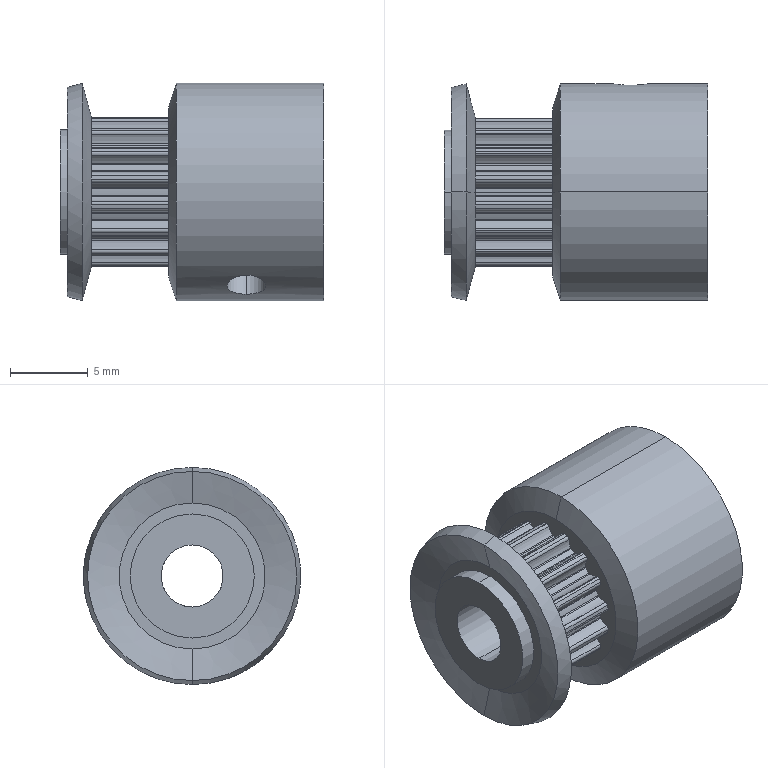Part | SolidWorks | features BaseBody 1 | 1 solid | 183 faces | box 17 x 14 x 14 mm | volume 1770 mm3 | cylinder 155 | plane 20 | cone 8 | commonest cylinder face diameters 0.38 x40 0.2 x36 2.65 x36 8.16 x17 9.68 x16 2.459 x4